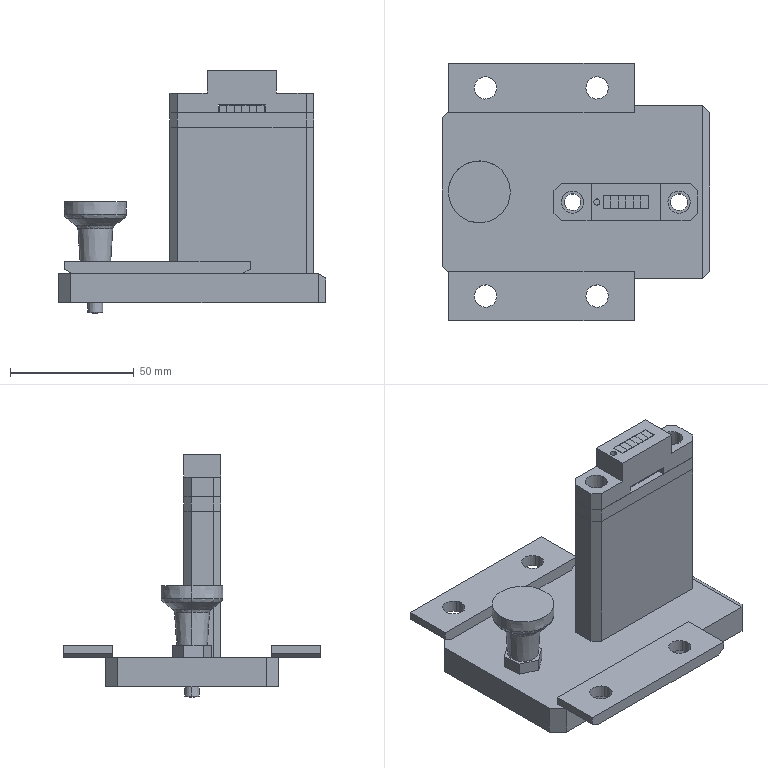Part | CATIA | 13 solids | 191 faces | box 108 x 104 x 97.9 mm | volume 166233 mm3 | plane 139 | cylinder 28 | spline 20 | cone 4 | commonest cylinder face diameters 9 x20 6.8 x4 2.5 x2 10.5 x2